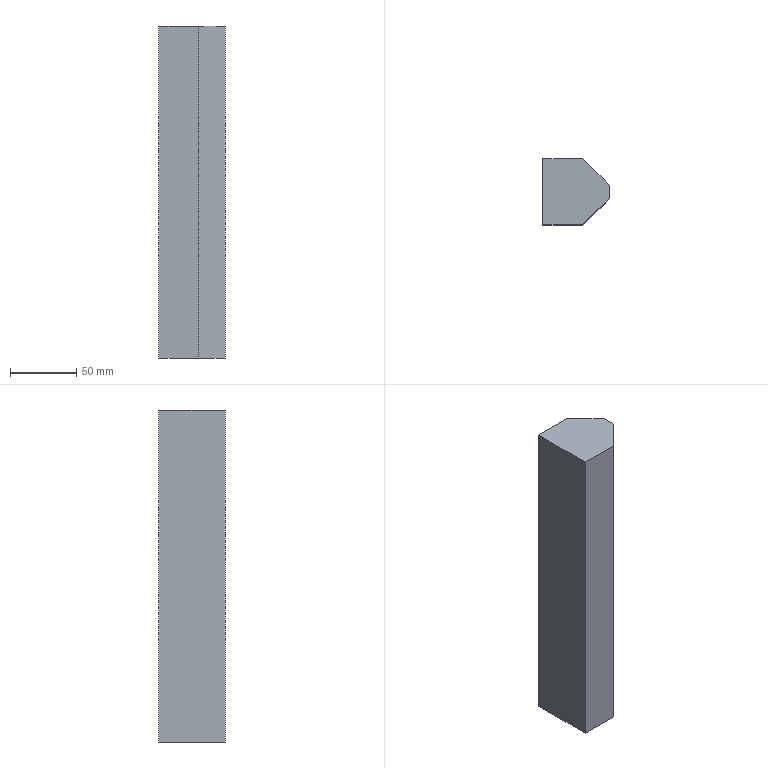Part | SolidWorks | features Chamfer 1, Extrusion 1 | 1 solid | 8 faces | box 50 x 50 x 250 mm | volume 525000 mm3 | plane 8
STEP:
#1=CARTESIAN_POINT('',(5.,-25.,125.));
#2=VERTEX_POINT('',#1);
#3=CARTESIAN_POINT('',(-25.,-25.,125.));
#4=VERTEX_POINT('',#3);
#5=CARTESIAN_POINT('',(25.,-25.,125.));
#6=DIRECTION('',(-1.,0.,0.));
#7=VECTOR('',#6,1000.);
#8=LINE('',#5,#7);
#9=EDGE_CURVE('',#2,#4,#8,.T.);
#10=ORIENTED_EDGE('',*,*,#9,.F.);
#11=CARTESIAN_POINT('',(25.,-5.,125.));
#12=VERTEX_POINT('',#11);
#13=CARTESIAN_POINT('',(25.,-5.,125.));
#14=DIRECTION('',(0.7071,0.7071,0.));
#15=VECTOR('',#14,1000.);
#16=LINE('',#13,#15);
#17=EDGE_CURVE('',#2,#12,#16,.T.);
#18=ORIENTED_EDGE('',*,*,#17,.T.);
#19=CARTESIAN_POINT('',(25.,5.,125.));
#20=VERTEX_POINT('',#19);
#21=CARTESIAN_POINT('',(25.,-25.,125.));
#22=DIRECTION('',(0.,-1.,0.));
#23=VECTOR('',#22,1000.);
#24=LINE('',#21,#23);
#25=EDGE_CURVE('',#20,#12,#24,.T.);
#26=ORIENTED_EDGE('',*,*,#25,.F.);
#27=CARTESIAN_POINT('',(5.,25.,125.));
#28=VERTEX_POINT('',#27);
#29=CARTESIAN_POINT('',(25.,5.,125.));
#30=DIRECTION('',(-0.7071,0.7071,0.));
#31=VECTOR('',#30,1000.);
#32=LINE('',#29,#31);
#33=EDGE_CURVE('',#20,#28,#32,.T.);
#34=ORIENTED_EDGE('',*,*,#33,.T.);
#35=CARTESIAN_POINT('',(-25.,25.,125.));
#36=VERTEX_POINT('',#35);
#37=CARTESIAN_POINT('',(25.,25.,125.));
#38=DIRECTION('',(-1.,0.,0.));
#39=VECTOR('',#38,1000.);
#40=LINE('',#37,#39);
#41=EDGE_CURVE('',#28,#36,#40,.T.);
#42=ORIENTED_EDGE('',*,*,#41,.T.);
#43=CARTESIAN_POINT('',(-25.,-25.,125.));
#44=DIRECTION('',(0.,-1.,0.));
#45=VECTOR('',#44,1000.);
#46=LINE('',#43,#45);
#47=EDGE_CURVE('',#36,#4,#46,.T.);
#48=ORIENTED_EDGE('',*,*,#47,.T.);
#49=EDGE_LOOP('',(#10,#18,#26,#34,#42,#48));
#50=FACE_OUTER_BOUND('',#49,.T.);
#51=CARTESIAN_POINT('',(25.,-25.,125.));
#52=DIRECTION('',(0.,0.,-1.));
#53=DIRECTION('',(-1.,0.,0.));
#54=AXIS2_PLACEMENT_3D('',#51,#52,#53);
#55=PLANE('',#54);
#56=ADVANCED_FACE('',(#50),#55,.F.);
#57=CARTESIAN_POINT('',(5.,-25.,-125.));
#58=VERTEX_POINT('',#57);
#59=CARTESIAN_POINT('',(-25.,-25.,-125.));
#60=VERTEX_POINT('',#59);
#61=CARTESIAN_POINT('',(25.,-25.,-125.));
#62=DIRECTION('',(-1.,0.,0.));
#63=VECTOR('',#62,1000.);
#64=LINE('',#61,#63);
#65=EDGE_CURVE('',#58,#60,#64,.T.);
#66=ORIENTED_EDGE('',*,*,#65,.F.);
#67=CARTESIAN_POINT('',(5.,-25.,125.));
#68=DIRECTION('',(0.,0.,1.));
#69=VECTOR('',#68,1000.);
#70=LINE('',#67,#69);
#71=EDGE_CURVE('',#58,#2,#70,.T.);
#72=ORIENTED_EDGE('',*,*,#71,.T.);
#73=ORIENTED_EDGE('',*,*,#9,.T.);
#74=CARTESIAN_POINT('',(-25.,-25.,-125.));
#75=DIRECTION('',(0.,0.,-1.));
#76=VECTOR('',#75,1000.);
#77=LINE('',#74,#76);
#78=EDGE_CURVE('',#4,#60,#77,.T.);
#79=ORIENTED_EDGE('',*,*,#78,.T.);
#80=EDGE_LOOP('',(#66,#72,#73,#79));
#81=FACE_OUTER_BOUND('',#80,.T.);
#82=CARTESIAN_POINT('',(25.,-25.,-125.));
#83=DIRECTION('',(0.,1.,0.));
#84=DIRECTION('',(0.,0.,1.));
#85=AXIS2_PLACEMENT_3D('',#82,#83,#84);
#86=PLANE('',#85);
#87=ADVANCED_FACE('',(#81),#86,.F.);
#88=CARTESIAN_POINT('',(25.,-5.,-125.));
#89=VERTEX_POINT('',#88);
#90=CARTESIAN_POINT('',(25.,5.,-125.));
#91=VERTEX_POINT('',#90);
#92=CARTESIAN_POINT('',(25.,-25.,-125.));
#93=DIRECTION('',(0.,1.,0.));
#94=VECTOR('',#93,1000.);
#95=LINE('',#92,#94);
#96=EDGE_CURVE('',#89,#91,#95,.T.);
#97=ORIENTED_EDGE('',*,*,#96,.F.);
#98=CARTESIAN_POINT('',(25.,-5.,-125.));
#99=DIRECTION('',(-0.7071,-0.7071,0.));
#100=VECTOR('',#99,1000.);
#101=LINE('',#98,#100);
#102=EDGE_CURVE('',#89,#58,#101,.T.);
#103=ORIENTED_EDGE('',*,*,#102,.T.);
#104=ORIENTED_EDGE('',*,*,#65,.T.);
#105=CARTESIAN_POINT('',(-25.,25.,-125.));
#106=VERTEX_POINT('',#105);
#107=CARTESIAN_POINT('',(-25.,-25.,-125.));
#108=DIRECTION('',(0.,1.,0.));
#109=VECTOR('',#108,1000.);
#110=LINE('',#107,#109);
#111=EDGE_CURVE('',#60,#106,#110,.T.);
#112=ORIENTED_EDGE('',*,*,#111,.T.);
#113=CARTESIAN_POINT('',(5.,25.,-125.));
#114=VERTEX_POINT('',#113);
#115=CARTESIAN_POINT('',(25.,25.,-125.));
#116=DIRECTION('',(-1.,0.,0.));
#117=VECTOR('',#116,1000.);
#118=LINE('',#115,#117);
#119=EDGE_CURVE('',#114,#106,#118,.T.);
#120=ORIENTED_EDGE('',*,*,#119,.F.);
#121=CARTESIAN_POINT('',(25.,5.,-125.));
#122=DIRECTION('',(0.7071,-0.7071,0.));
#123=VECTOR('',#122,1000.);
#124=LINE('',#121,#123);
#125=EDGE_CURVE('',#114,#91,#124,.T.);
#126=ORIENTED_EDGE('',*,*,#125,.T.);
#127=EDGE_LOOP('',(#97,#103,#104,#112,#120,#126));
#128=FACE_OUTER_BOUND('',#127,.T.);
#129=CARTESIAN_POINT('',(25.,-25.,-125.));
#130=DIRECTION('',(0.,0.,1.));
#131=DIRECTION('',(1.,0.,0.));
#132=AXIS2_PLACEMENT_3D('',#129,#130,#131);
#133=PLANE('',#132);
#134=ADVANCED_FACE('',(#128),#133,.F.);
#135=ORIENTED_EDGE('',*,*,#41,.F.);
#136=CARTESIAN_POINT('',(5.,25.,-125.));
#137=DIRECTION('',(0.,0.,-1.));
#138=VECTOR('',#137,1000.);
#139=LINE('',#136,#138);
#140=EDGE_CURVE('',#28,#114,#139,.T.);
#141=ORIENTED_EDGE('',*,*,#140,.T.);
#142=ORIENTED_EDGE('',*,*,#119,.T.);
#143=CARTESIAN_POINT('',(-25.,25.,-125.));
#144=DIRECTION('',(0.,0.,1.));
#145=VECTOR('',#144,1000.);
#146=LINE('',#143,#145);
#147=EDGE_CURVE('',#106,#36,#146,.T.);
#148=ORIENTED_EDGE('',*,*,#147,.T.);
#149=EDGE_LOOP('',(#135,#141,#142,#148));
#150=FACE_OUTER_BOUND('',#149,.T.);
#151=CARTESIAN_POINT('',(25.,25.,-125.));
#152=DIRECTION('',(0.,-1.,0.));
#153=DIRECTION('',(0.,0.,-1.));
#154=AXIS2_PLACEMENT_3D('',#151,#152,#153);
#155=PLANE('',#154);
#156=ADVANCED_FACE('',(#150),#155,.F.);
#157=ORIENTED_EDGE('',*,*,#25,.T.);
#158=CARTESIAN_POINT('',(25.,-5.,-125.));
#159=DIRECTION('',(0.,0.,-1.));
#160=VECTOR('',#159,1000.);
#161=LINE('',#158,#160);
#162=EDGE_CURVE('',#12,#89,#161,.T.);
#163=ORIENTED_EDGE('',*,*,#162,.T.);
#164=ORIENTED_EDGE('',*,*,#96,.T.);
#165=CARTESIAN_POINT('',(25.,5.,125.));
#166=DIRECTION('',(0.,0.,1.));
#167=VECTOR('',#166,1000.);
#168=LINE('',#165,#167);
#169=EDGE_CURVE('',#91,#20,#168,.T.);
#170=ORIENTED_EDGE('',*,*,#169,.T.);
#171=EDGE_LOOP('',(#157,#163,#164,#170));
#172=FACE_OUTER_BOUND('',#171,.T.);
#173=CARTESIAN_POINT('',(25.,0.,0.));
#174=DIRECTION('',(1.,0.,0.));
#175=DIRECTION('',(0.,0.,-1.));
#176=AXIS2_PLACEMENT_3D('',#173,#174,#175);
#177=PLANE('',#176);
#178=ADVANCED_FACE('',(#172),#177,.T.);
#179=ORIENTED_EDGE('',*,*,#47,.F.);
#180=ORIENTED_EDGE('',*,*,#147,.F.);
#181=ORIENTED_EDGE('',*,*,#111,.F.);
#182=ORIENTED_EDGE('',*,*,#78,.F.);
#183=EDGE_LOOP('',(#179,#180,#181,#182));
#184=FACE_OUTER_BOUND('',#183,.T.);
#185=CARTESIAN_POINT('',(-25.,0.,0.));
#186=DIRECTION('',(1.,0.,0.));
#187=DIRECTION('',(0.,0.,-1.));
#188=AXIS2_PLACEMENT_3D('',#185,#186,#187);
#189=PLANE('',#188);
#190=ADVANCED_FACE('',(#184),#189,.F.);
#191=ORIENTED_EDGE('',*,*,#17,.F.);
#192=ORIENTED_EDGE('',*,*,#71,.F.);
#193=ORIENTED_EDGE('',*,*,#102,.F.);
#194=ORIENTED_EDGE('',*,*,#162,.F.);
#195=EDGE_LOOP('',(#191,#192,#193,#194));
#196=FACE_OUTER_BOUND('',#195,.T.);
#197=CARTESIAN_POINT('',(25.,-5.,0.));
#198=DIRECTION('',(0.7071,-0.7071,0.));
#199=DIRECTION('',(0.,0.,1.));
#200=AXIS2_PLACEMENT_3D('',#197,#198,#199);
#201=PLANE('',#200);
#202=ADVANCED_FACE('',(#196),#201,.T.);
#203=ORIENTED_EDGE('',*,*,#125,.F.);
#204=ORIENTED_EDGE('',*,*,#140,.F.);
#205=ORIENTED_EDGE('',*,*,#33,.F.);
#206=ORIENTED_EDGE('',*,*,#169,.F.);
#207=EDGE_LOOP('',(#203,#204,#205,#206));
#208=FACE_OUTER_BOUND('',#207,.T.);
#209=CARTESIAN_POINT('',(25.,5.,0.));
#210=DIRECTION('',(0.7071,0.7071,0.));
#211=DIRECTION('',(0.,0.,-1.));
#212=AXIS2_PLACEMENT_3D('',#209,#210,#211);
#213=PLANE('',#212);
#214=ADVANCED_FACE('',(#208),#213,.T.);
#215=CLOSED_SHELL('',(#56,#87,#134,#156,#178,#190,#202,#214));
#216=MANIFOLD_SOLID_BREP('',#215);
#217=CARTESIAN_POINT('',(0.,0.,0.));
#218=DIRECTION('',(0.,0.,1.));
#219=DIRECTION('',(1.,0.,0.));
#220=AXIS2_PLACEMENT_3D('',#217,#218,#219);
#221=(LENGTH_UNIT()NAMED_UNIT(*)SI_UNIT(.MILLI.,.METRE.));
#222=UNCERTAINTY_MEASURE_WITH_UNIT(LENGTH_MEASURE(0.00001),#221,'','');
#223=(NAMED_UNIT(*)PLANE_ANGLE_UNIT()SI_UNIT($,.RADIAN.));
#224=(NAMED_UNIT(*)SI_UNIT($,.STERADIAN.)SOLID_ANGLE_UNIT());
#225=(GEOMETRIC_REPRESENTATION_CONTEXT(3)GLOBAL_UNCERTAINTY_ASSIGNED_CONTEXT((#222))GLOBAL_UNIT_ASSIGNED_CONTEXT((#221,#223,#224))REPRESENTATION_CONTEXT('',''));
#226=ADVANCED_BREP_SHAPE_REPRESENTATION('',(#216,#220),#225);